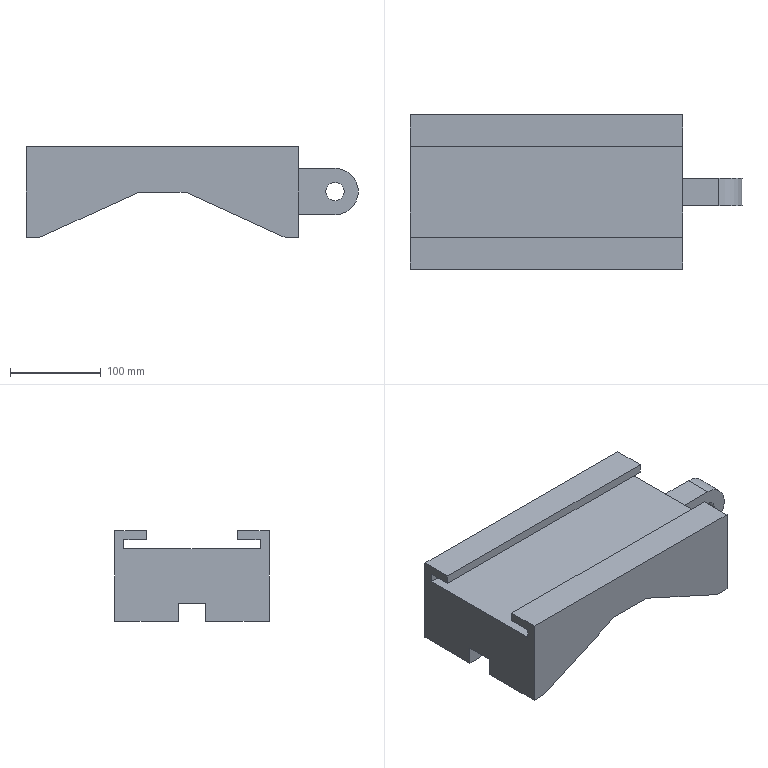Part | SolidWorks | features ICE 5, MirrorPattern 2, Extrusion 1 | 1 solid | 37 faces | box 365.5 x 170 x 100 mm | volume 2892418 mm3 | plane 34 | cylinder 3 | commonest cylinder face diameters 20 x2 51 x1
STEP:
#1=CARTESIAN_POINT('',(190.,15.,-29.5));
#2=VERTEX_POINT('',#1);
#3=CARTESIAN_POINT('',(190.,15.,-9.5));
#4=VERTEX_POINT('',#3);
#5=CARTESIAN_POINT('',(190.,15.,-19.5));
#6=DIRECTION('',(0.,1.,0.));
#7=DIRECTION('',(0.,0.,1.));
#8=AXIS2_PLACEMENT_3D('',#5,#6,#7);
#9=CIRCLE('',#8,10.);
#10=EDGE_CURVE('',#2,#4,#9,.T.);
#11=ORIENTED_EDGE('',*,*,#10,.T.);
#12=CARTESIAN_POINT('',(190.,-15.,-9.5));
#13=VERTEX_POINT('',#12);
#14=CARTESIAN_POINT('',(190.,15.,-9.5));
#15=DIRECTION('',(0.,-1.,0.));
#16=VECTOR('',#15,1000.);
#17=LINE('',#14,#16);
#18=EDGE_CURVE('',#4,#13,#17,.T.);
#19=ORIENTED_EDGE('',*,*,#18,.T.);
#20=CARTESIAN_POINT('',(190.,-15.,-29.5));
#21=VERTEX_POINT('',#20);
#22=CARTESIAN_POINT('',(190.,-15.,-19.5));
#23=DIRECTION('',(0.,1.,0.));
#24=DIRECTION('',(0.,0.,1.));
#25=AXIS2_PLACEMENT_3D('',#22,#23,#24);
#26=CIRCLE('',#25,10.);
#27=EDGE_CURVE('',#21,#13,#26,.T.);
#28=ORIENTED_EDGE('',*,*,#27,.F.);
#29=CARTESIAN_POINT('',(190.,15.,-29.5));
#30=DIRECTION('',(0.,-1.,0.));
#31=VECTOR('',#30,1000.);
#32=LINE('',#29,#31);
#33=EDGE_CURVE('',#2,#21,#32,.T.);
#34=ORIENTED_EDGE('',*,*,#33,.F.);
#35=EDGE_LOOP('',(#11,#19,#28,#34));
#36=FACE_OUTER_BOUND('',#35,.T.);
#37=CARTESIAN_POINT('',(190.,15.,-19.5));
#38=DIRECTION('',(0.,-1.,0.));
#39=DIRECTION('',(0.,0.,-1.));
#40=AXIS2_PLACEMENT_3D('',#37,#38,#39);
#41=CYLINDRICAL_SURFACE('',#40,10.);
#42=ADVANCED_FACE('',(#36),#41,.F.);
#43=CARTESIAN_POINT('',(150.,-15.,-70.));
#44=VERTEX_POINT('',#43);
#45=CARTESIAN_POINT('',(150.,-85.,-70.));
#46=VERTEX_POINT('',#45);
#47=CARTESIAN_POINT('',(150.,85.,-70.));
#48=DIRECTION('',(0.,-1.,0.));
#49=VECTOR('',#48,1000.);
#50=LINE('',#47,#49);
#51=EDGE_CURVE('',#44,#46,#50,.T.);
#52=ORIENTED_EDGE('',*,*,#51,.F.);
#53=CARTESIAN_POINT('',(150.,-15.,-50.));
#54=VERTEX_POINT('',#53);
#55=CARTESIAN_POINT('',(150.,-15.,-50.));
#56=DIRECTION('',(0.,0.,1.));
#57=VECTOR('',#56,1000.);
#58=LINE('',#55,#57);
#59=EDGE_CURVE('',#44,#54,#58,.T.);
#60=ORIENTED_EDGE('',*,*,#59,.T.);
#61=CARTESIAN_POINT('',(150.,15.,-50.));
#62=VERTEX_POINT('',#61);
#63=CARTESIAN_POINT('',(150.,-15.,-50.));
#64=DIRECTION('',(0.,1.,0.));
#65=VECTOR('',#64,1000.);
#66=LINE('',#63,#65);
#67=EDGE_CURVE('',#54,#62,#66,.T.);
#68=ORIENTED_EDGE('',*,*,#67,.T.);
#69=CARTESIAN_POINT('',(150.,15.,-70.));
#70=VERTEX_POINT('',#69);
#71=CARTESIAN_POINT('',(150.,15.,-50.));
#72=DIRECTION('',(0.,0.,1.));
#73=VECTOR('',#72,1000.);
#74=LINE('',#71,#73);
#75=EDGE_CURVE('',#70,#62,#74,.T.);
#76=ORIENTED_EDGE('',*,*,#75,.F.);
#77=CARTESIAN_POINT('',(150.,85.,-70.));
#78=VERTEX_POINT('',#77);
#79=CARTESIAN_POINT('',(150.,85.,-70.));
#80=DIRECTION('',(0.,-1.,0.));
#81=VECTOR('',#80,1000.);
#82=LINE('',#79,#81);
#83=EDGE_CURVE('',#78,#70,#82,.T.);
#84=ORIENTED_EDGE('',*,*,#83,.F.);
#85=CARTESIAN_POINT('',(150.,85.,30.));
#86=VERTEX_POINT('',#85);
#87=CARTESIAN_POINT('',(150.,85.,10.));
#88=DIRECTION('',(0.,0.,-1.));
#89=VECTOR('',#88,1000.);
#90=LINE('',#87,#89);
#91=EDGE_CURVE('',#86,#78,#90,.T.);
#92=ORIENTED_EDGE('',*,*,#91,.F.);
#93=CARTESIAN_POINT('',(150.,50.,30.));
#94=VERTEX_POINT('',#93);
#95=CARTESIAN_POINT('',(150.,85.,30.));
#96=DIRECTION('',(0.,1.,0.));
#97=VECTOR('',#96,1000.);
#98=LINE('',#95,#97);
#99=EDGE_CURVE('',#94,#86,#98,.T.);
#100=ORIENTED_EDGE('',*,*,#99,.F.);
#101=CARTESIAN_POINT('',(150.,50.,20.));
#102=VERTEX_POINT('',#101);
#103=CARTESIAN_POINT('',(150.,50.,30.));
#104=DIRECTION('',(0.,0.,1.));
#105=VECTOR('',#104,1000.);
#106=LINE('',#103,#105);
#107=EDGE_CURVE('',#102,#94,#106,.T.);
#108=ORIENTED_EDGE('',*,*,#107,.F.);
#109=CARTESIAN_POINT('',(150.,75.,20.));
#110=VERTEX_POINT('',#109);
#111=CARTESIAN_POINT('',(150.,50.,20.));
#112=DIRECTION('',(0.,1.,0.));
#113=VECTOR('',#112,1000.);
#114=LINE('',#111,#113);
#115=EDGE_CURVE('',#102,#110,#114,.T.);
#116=ORIENTED_EDGE('',*,*,#115,.T.);
#117=CARTESIAN_POINT('',(150.,75.,10.));
#118=VERTEX_POINT('',#117);
#119=CARTESIAN_POINT('',(150.,75.,30.));
#120=DIRECTION('',(0.,0.,-1.));
#121=VECTOR('',#120,1000.);
#122=LINE('',#119,#121);
#123=EDGE_CURVE('',#110,#118,#122,.T.);
#124=ORIENTED_EDGE('',*,*,#123,.T.);
#125=CARTESIAN_POINT('',(150.,-75.,10.));
#126=VERTEX_POINT('',#125);
#127=CARTESIAN_POINT('',(150.,85.,10.));
#128=DIRECTION('',(0.,1.,0.));
#129=VECTOR('',#128,1000.);
#130=LINE('',#127,#129);
#131=EDGE_CURVE('',#126,#118,#130,.T.);
#132=ORIENTED_EDGE('',*,*,#131,.F.);
#133=CARTESIAN_POINT('',(150.,-75.,20.));
#134=VERTEX_POINT('',#133);
#135=CARTESIAN_POINT('',(150.,-75.,30.));
#136=DIRECTION('',(0.,0.,-1.));
#137=VECTOR('',#136,1000.);
#138=LINE('',#135,#137);
#139=EDGE_CURVE('',#134,#126,#138,.T.);
#140=ORIENTED_EDGE('',*,*,#139,.F.);
#141=CARTESIAN_POINT('',(150.,-50.,20.));
#142=VERTEX_POINT('',#141);
#143=CARTESIAN_POINT('',(150.,-50.,20.));
#144=DIRECTION('',(0.,-1.,0.));
#145=VECTOR('',#144,1000.);
#146=LINE('',#143,#145);
#147=EDGE_CURVE('',#142,#134,#146,.T.);
#148=ORIENTED_EDGE('',*,*,#147,.F.);
#149=CARTESIAN_POINT('',(150.,-50.,30.));
#150=VERTEX_POINT('',#149);
#151=CARTESIAN_POINT('',(150.,-50.,30.));
#152=DIRECTION('',(0.,0.,1.));
#153=VECTOR('',#152,1000.);
#154=LINE('',#151,#153);
#155=EDGE_CURVE('',#142,#150,#154,.T.);
#156=ORIENTED_EDGE('',*,*,#155,.T.);
#157=CARTESIAN_POINT('',(150.,-85.,30.));
#158=VERTEX_POINT('',#157);
#159=CARTESIAN_POINT('',(150.,-85.,30.));
#160=DIRECTION('',(0.,1.,0.));
#161=VECTOR('',#160,1000.);
#162=LINE('',#159,#161);
#163=EDGE_CURVE('',#158,#150,#162,.T.);
#164=ORIENTED_EDGE('',*,*,#163,.F.);
#165=CARTESIAN_POINT('',(150.,-85.,10.));
#166=DIRECTION('',(0.,0.,-1.));
#167=VECTOR('',#166,1000.);
#168=LINE('',#165,#167);
#169=EDGE_CURVE('',#158,#46,#168,.T.);
#170=ORIENTED_EDGE('',*,*,#169,.T.);
#171=EDGE_LOOP('',(#52,#60,#68,#76,#84,#92,#100,#108,#116,#124,#132,#140,#148,#156,#164,#170));
#172=FACE_OUTER_BOUND('',#171,.T.);
#173=CARTESIAN_POINT('',(150.,15.,6.));
#174=VERTEX_POINT('',#173);
#175=CARTESIAN_POINT('',(150.,-15.,6.));
#176=VERTEX_POINT('',#175);
#177=CARTESIAN_POINT('',(150.,15.,6.));
#178=DIRECTION('',(0.,-1.,0.));
#179=VECTOR('',#178,1000.);
#180=LINE('',#177,#179);
#181=EDGE_CURVE('',#174,#176,#180,.T.);
#182=ORIENTED_EDGE('',*,*,#181,.F.);
#183=CARTESIAN_POINT('',(150.,15.,-45.));
#184=VERTEX_POINT('',#183);
#185=CARTESIAN_POINT('',(150.,15.,6.));
#186=DIRECTION('',(0.,0.,1.));
#187=VECTOR('',#186,1000.);
#188=LINE('',#185,#187);
#189=EDGE_CURVE('',#184,#174,#188,.T.);
#190=ORIENTED_EDGE('',*,*,#189,.F.);
#191=CARTESIAN_POINT('',(150.,-15.,-45.));
#192=VERTEX_POINT('',#191);
#193=CARTESIAN_POINT('',(150.,15.,-45.));
#194=DIRECTION('',(0.,-1.,0.));
#195=VECTOR('',#194,1000.);
#196=LINE('',#193,#195);
#197=EDGE_CURVE('',#184,#192,#196,.T.);
#198=ORIENTED_EDGE('',*,*,#197,.T.);
#199=CARTESIAN_POINT('',(150.,-15.,6.));
#200=DIRECTION('',(0.,0.,1.));
#201=VECTOR('',#200,1000.);
#202=LINE('',#199,#201);
#203=EDGE_CURVE('',#192,#176,#202,.T.);
#204=ORIENTED_EDGE('',*,*,#203,.T.);
#205=EDGE_LOOP('',(#182,#190,#198,#204));
#206=FACE_BOUND('',#205,.T.);
#207=CARTESIAN_POINT('',(150.,85.,10.));
#208=DIRECTION('',(-1.,0.,0.));
#209=DIRECTION('',(0.,-1.,0.));
#210=AXIS2_PLACEMENT_3D('',#207,#208,#209);
#211=PLANE('',#210);
#212=ADVANCED_FACE('',(#172,#206),#211,.F.);
#213=CARTESIAN_POINT('',(25.,85.,-20.));
#214=VERTEX_POINT('',#213);
#215=CARTESIAN_POINT('',(25.,15.,-20.));
#216=VERTEX_POINT('',#215);
#217=CARTESIAN_POINT('',(25.,85.,-20.));
#218=DIRECTION('',(0.,-1.,0.));
#219=VECTOR('',#218,1000.);
#220=LINE('',#217,#219);
#221=EDGE_CURVE('',#214,#216,#220,.T.);
#222=ORIENTED_EDGE('',*,*,#221,.T.);
#223=CARTESIAN_POINT('',(-25.,15.,-20.));
#224=VERTEX_POINT('',#223);
#225=CARTESIAN_POINT('',(-25.,15.,-20.));
#226=DIRECTION('',(-1.,0.,0.));
#227=VECTOR('',#226,1000.);
#228=LINE('',#225,#227);
#229=EDGE_CURVE('',#216,#224,#228,.T.);
#230=ORIENTED_EDGE('',*,*,#229,.T.);
#231=CARTESIAN_POINT('',(-25.,85.,-20.));
#232=VERTEX_POINT('',#231);
#233=CARTESIAN_POINT('',(-25.,85.,-20.));
#234=DIRECTION('',(0.,-1.,0.));
#235=VECTOR('',#234,1000.);
#236=LINE('',#233,#235);
#237=EDGE_CURVE('',#232,#224,#236,.T.);
#238=ORIENTED_EDGE('',*,*,#237,.F.);
#239=CARTESIAN_POINT('',(-25.,85.,-20.));
#240=DIRECTION('',(-1.,0.,0.));
#241=VECTOR('',#240,1000.);
#242=LINE('',#239,#241);
#243=EDGE_CURVE('',#214,#232,#242,.T.);
#244=ORIENTED_EDGE('',*,*,#243,.F.);
#245=EDGE_LOOP('',(#222,#230,#238,#244));
#246=FACE_OUTER_BOUND('',#245,.T.);
#247=CARTESIAN_POINT('',(-25.,85.,-20.));
#248=DIRECTION('',(0.,0.,1.));
#249=DIRECTION('',(1.,0.,0.));
#250=AXIS2_PLACEMENT_3D('',#247,#248,#249);
#251=PLANE('',#250);
#252=ADVANCED_FACE('',(#246),#251,.F.);
#253=ORIENTED_EDGE('',*,*,#83,.T.);
#254=CARTESIAN_POINT('',(135.,15.,-70.));
#255=VERTEX_POINT('',#254);
#256=CARTESIAN_POINT('',(150.,15.,-70.));
#257=DIRECTION('',(1.,0.,0.));
#258=VECTOR('',#257,1000.);
#259=LINE('',#256,#258);
#260=EDGE_CURVE('',#255,#70,#259,.T.);
#261=ORIENTED_EDGE('',*,*,#260,.F.);
#262=CARTESIAN_POINT('',(135.,85.,-70.));
#263=VERTEX_POINT('',#262);
#264=CARTESIAN_POINT('',(135.,85.,-70.));
#265=DIRECTION('',(0.,-1.,0.));
#266=VECTOR('',#265,1000.);
#267=LINE('',#264,#266);
#268=EDGE_CURVE('',#263,#255,#267,.T.);
#269=ORIENTED_EDGE('',*,*,#268,.F.);
#270=CARTESIAN_POINT('',(150.,85.,-70.));
#271=DIRECTION('',(1.,0.,0.));
#272=VECTOR('',#271,1000.);
#273=LINE('',#270,#272);
#274=EDGE_CURVE('',#263,#78,#273,.T.);
#275=ORIENTED_EDGE('',*,*,#274,.T.);
#276=EDGE_LOOP('',(#253,#261,#269,#275));
#277=FACE_OUTER_BOUND('',#276,.T.);
#278=CARTESIAN_POINT('',(150.,85.,-70.));
#279=DIRECTION('',(0.,0.,-1.));
#280=DIRECTION('',(-1.,0.,0.));
#281=AXIS2_PLACEMENT_3D('',#278,#279,#280);
#282=PLANE('',#281);
#283=ADVANCED_FACE('',(#277),#282,.T.);
#284=ORIENTED_EDGE('',*,*,#268,.T.);
#285=CARTESIAN_POINT('',(135.,15.,-70.));
#286=DIRECTION('',(0.9104,0.,-0.4138));
#287=VECTOR('',#286,1000.);
#288=LINE('',#285,#287);
#289=EDGE_CURVE('',#216,#255,#288,.T.);
#290=ORIENTED_EDGE('',*,*,#289,.F.);
#291=ORIENTED_EDGE('',*,*,#221,.F.);
#292=CARTESIAN_POINT('',(135.,85.,-70.));
#293=DIRECTION('',(0.9104,0.,-0.4138));
#294=VECTOR('',#293,1000.);
#295=LINE('',#292,#294);
#296=EDGE_CURVE('',#214,#263,#295,.T.);
#297=ORIENTED_EDGE('',*,*,#296,.T.);
#298=EDGE_LOOP('',(#284,#290,#291,#297));
#299=FACE_OUTER_BOUND('',#298,.T.);
#300=CARTESIAN_POINT('',(135.,85.,-70.));
#301=DIRECTION('',(-0.4138,0.,-0.9104));
#302=DIRECTION('',(-0.9104,0.,0.4138));
#303=AXIS2_PLACEMENT_3D('',#300,#301,#302);
#304=PLANE('',#303);
#305=ADVANCED_FACE('',(#299),#304,.T.);
#306=CARTESIAN_POINT('',(-135.,15.,-70.));
#307=VERTEX_POINT('',#306);
#308=CARTESIAN_POINT('',(-135.,15.,-70.));
#309=DIRECTION('',(-0.9104,0.,-0.4138));
#310=VECTOR('',#309,1000.);
#311=LINE('',#308,#310);
#312=EDGE_CURVE('',#224,#307,#311,.T.);
#313=ORIENTED_EDGE('',*,*,#312,.T.);
#314=CARTESIAN_POINT('',(-135.,85.,-70.));
#315=VERTEX_POINT('',#314);
#316=CARTESIAN_POINT('',(-135.,85.,-70.));
#317=DIRECTION('',(0.,-1.,0.));
#318=VECTOR('',#317,1000.);
#319=LINE('',#316,#318);
#320=EDGE_CURVE('',#315,#307,#319,.T.);
#321=ORIENTED_EDGE('',*,*,#320,.F.);
#322=CARTESIAN_POINT('',(-135.,85.,-70.));
#323=DIRECTION('',(-0.9104,0.,-0.4138));
#324=VECTOR('',#323,1000.);
#325=LINE('',#322,#324);
#326=EDGE_CURVE('',#232,#315,#325,.T.);
#327=ORIENTED_EDGE('',*,*,#326,.F.);
#328=ORIENTED_EDGE('',*,*,#237,.T.);
#329=EDGE_LOOP('',(#313,#321,#327,#328));
#330=FACE_OUTER_BOUND('',#329,.T.);
#331=CARTESIAN_POINT('',(-135.,85.,-70.));
#332=DIRECTION('',(-0.4138,0.,0.9104));
#333=DIRECTION('',(0.9104,0.,0.4138));
#334=AXIS2_PLACEMENT_3D('',#331,#332,#333);
#335=PLANE('',#334);
#336=ADVANCED_FACE('',(#330),#335,.F.);
#337=CARTESIAN_POINT('',(-150.,15.,-70.));
#338=VERTEX_POINT('',#337);
#339=CARTESIAN_POINT('',(-150.,15.,-70.));
#340=DIRECTION('',(-1.,0.,0.));
#341=VECTOR('',#340,1000.);
#342=LINE('',#339,#341);
#343=EDGE_CURVE('',#307,#338,#342,.T.);
#344=ORIENTED_EDGE('',*,*,#343,.T.);
#345=CARTESIAN_POINT('',(-150.,85.,-70.));
#346=VERTEX_POINT('',#345);
#347=CARTESIAN_POINT('',(-150.,85.,-70.));
#348=DIRECTION('',(0.,-1.,0.));
#349=VECTOR('',#348,1000.);
#350=LINE('',#347,#349);
#351=EDGE_CURVE('',#346,#338,#350,.T.);
#352=ORIENTED_EDGE('',*,*,#351,.F.);
#353=CARTESIAN_POINT('',(-150.,85.,-70.));
#354=DIRECTION('',(-1.,0.,0.));
#355=VECTOR('',#354,1000.);
#356=LINE('',#353,#355);
#357=EDGE_CURVE('',#315,#346,#356,.T.);
#358=ORIENTED_EDGE('',*,*,#357,.F.);
#359=ORIENTED_EDGE('',*,*,#320,.T.);
#360=EDGE_LOOP('',(#344,#352,#358,#359));
#361=FACE_OUTER_BOUND('',#360,.T.);
#362=CARTESIAN_POINT('',(-150.,85.,-70.));
#363=DIRECTION('',(0.,0.,1.));
#364=DIRECTION('',(1.,0.,0.));
#365=AXIS2_PLACEMENT_3D('',#362,#363,#364);
#366=PLANE('',#365);
#367=ADVANCED_FACE('',(#361),#366,.F.);
#368=CARTESIAN_POINT('',(-25.,15.,0.));
#369=VERTEX_POINT('',#368);
#370=CARTESIAN_POINT('',(25.,15.,0.));
#371=VERTEX_POINT('',#370);
#372=CARTESIAN_POINT('',(0.,15.,0.));
#373=DIRECTION('',(1.,0.,0.));
#374=VECTOR('',#373,1000.);
#375=LINE('',#372,#374);
#376=EDGE_CURVE('',#369,#371,#375,.T.);
#377=ORIENTED_EDGE('',*,*,#376,.T.);
#378=CARTESIAN_POINT('',(25.,-15.,0.));
#379=VERTEX_POINT('',#378);
#380=CARTESIAN_POINT('',(25.,-15.,0.));
#381=DIRECTION('',(0.,1.,0.));
#382=VECTOR('',#381,1000.);
#383=LINE('',#380,#382);
#384=EDGE_CURVE('',#379,#371,#383,.T.);
#385=ORIENTED_EDGE('',*,*,#384,.F.);
#386=CARTESIAN_POINT('',(-25.,-15.,0.));
#387=VERTEX_POINT('',#386);
#388=CARTESIAN_POINT('',(0.,-15.,0.));
#389=DIRECTION('',(1.,0.,0.));
#390=VECTOR('',#389,1000.);
#391=LINE('',#388,#390);
#392=EDGE_CURVE('',#387,#379,#391,.T.);
#393=ORIENTED_EDGE('',*,*,#392,.F.);
#394=CARTESIAN_POINT('',(-25.,-15.,0.));
#395=DIRECTION('',(0.,1.,0.));
#396=VECTOR('',#395,1000.);
#397=LINE('',#394,#396);
#398=EDGE_CURVE('',#387,#369,#397,.T.);
#399=ORIENTED_EDGE('',*,*,#398,.T.);
#400=EDGE_LOOP('',(#377,#385,#393,#399));
#401=FACE_OUTER_BOUND('',#400,.T.);
#402=CARTESIAN_POINT('',(0.,0.,0.));
#403=DIRECTION('',(0.,0.,1.));
#404=DIRECTION('',(1.,0.,0.));
#405=AXIS2_PLACEMENT_3D('',#402,#403,#404);
#406=PLANE('',#405);
#407=ADVANCED_FACE('',(#401),#406,.F.);
#408=CARTESIAN_POINT('',(-150.,75.,20.));
#409=VERTEX_POINT('',#408);
#410=CARTESIAN_POINT('',(-150.,75.,20.));
#411=DIRECTION('',(1.,0.,0.));
#412=VECTOR('',#411,1000.);
#413=LINE('',#410,#412);
#414=EDGE_CURVE('',#409,#110,#413,.T.);
#415=ORIENTED_EDGE('',*,*,#414,.F.);
#416=CARTESIAN_POINT('',(-150.,75.,10.));
#417=VERTEX_POINT('',#416);
#418=CARTESIAN_POINT('',(-150.,75.,30.));
#419=DIRECTION('',(0.,0.,-1.));
#420=VECTOR('',#419,1000.);
#421=LINE('',#418,#420);
#422=EDGE_CURVE('',#409,#417,#421,.T.);
#423=ORIENTED_EDGE('',*,*,#422,.T.);
#424=CARTESIAN_POINT('',(-150.,75.,10.));
#425=DIRECTION('',(1.,0.,0.));
#426=VECTOR('',#425,1000.);
#427=LINE('',#424,#426);
#428=EDGE_CURVE('',#417,#118,#427,.T.);
#429=ORIENTED_EDGE('',*,*,#428,.T.);
#430=ORIENTED_EDGE('',*,*,#123,.F.);
#431=EDGE_LOOP('',(#415,#423,#429,#430));
#432=FACE_OUTER_BOUND('',#431,.T.);
#433=CARTESIAN_POINT('',(-150.,75.,30.));
#434=DIRECTION('',(0.,1.,0.));
#435=DIRECTION('',(-1.,0.,0.));
#436=AXIS2_PLACEMENT_3D('',#433,#434,#435);
#437=PLANE('',#436);
#438=ADVANCED_FACE('',(#432),#437,.F.);
#439=CARTESIAN_POINT('',(-150.,-75.,10.));
#440=VERTEX_POINT('',#439);
#441=CARTESIAN_POINT('',(-150.,85.,10.));
#442=DIRECTION('',(0.,-1.,0.));
#443=VECTOR('',#442,1000.);
#444=LINE('',#441,#443);
#445=EDGE_CURVE('',#417,#440,#444,.T.);
#446=ORIENTED_EDGE('',*,*,#445,.T.);
#447=CARTESIAN_POINT('',(-150.,-75.,10.));
#448=DIRECTION('',(-1.,0.,0.));
#449=VECTOR('',#448,1000.);
#450=LINE('',#447,#449);
#451=EDGE_CURVE('',#126,#440,#450,.T.);
#452=ORIENTED_EDGE('',*,*,#451,.F.);
#453=ORIENTED_EDGE('',*,*,#131,.T.);
#454=ORIENTED_EDGE('',*,*,#428,.F.);
#455=EDGE_LOOP('',(#446,#452,#453,#454));
#456=FACE_OUTER_BOUND('',#455,.T.);
#457=CARTESIAN_POINT('',(0.,0.,10.));
#458=DIRECTION('',(0.,0.,1.));
#459=DIRECTION('',(1.,0.,0.));
#460=AXIS2_PLACEMENT_3D('',#457,#458,#459);
#461=PLANE('',#460);
#462=ADVANCED_FACE('',(#456),#461,.T.);
#463=ORIENTED_EDGE('',*,*,#91,.T.);
#464=ORIENTED_EDGE('',*,*,#274,.F.);
#465=ORIENTED_EDGE('',*,*,#296,.F.);
#466=ORIENTED_EDGE('',*,*,#243,.T.);
#467=ORIENTED_EDGE('',*,*,#326,.T.);
#468=ORIENTED_EDGE('',*,*,#357,.T.);
#469=CARTESIAN_POINT('',(-150.,85.,30.));
#470=VERTEX_POINT('',#469);
#471=CARTESIAN_POINT('',(-150.,85.,10.));
#472=DIRECTION('',(0.,0.,-1.));
#473=VECTOR('',#472,1000.);
#474=LINE('',#471,#473);
#475=EDGE_CURVE('',#470,#346,#474,.T.);
#476=ORIENTED_EDGE('',*,*,#475,.F.);
#477=CARTESIAN_POINT('',(-150.,85.,30.));
#478=DIRECTION('',(-1.,0.,0.));
#479=VECTOR('',#478,1000.);
#480=LINE('',#477,#479);
#481=EDGE_CURVE('',#86,#470,#480,.T.);
#482=ORIENTED_EDGE('',*,*,#481,.F.);
#483=EDGE_LOOP('',(#463,#464,#465,#466,#467,#468,#476,#482));
#484=FACE_OUTER_BOUND('',#483,.T.);
#485=CARTESIAN_POINT('',(-150.,85.,10.));
#486=DIRECTION('',(0.,-1.,0.));
#487=DIRECTION('',(0.,0.,-1.));
#488=AXIS2_PLACEMENT_3D('',#485,#486,#487);
#489=PLANE('',#488);
#490=ADVANCED_FACE('',(#484),#489,.F.);
#491=CARTESIAN_POINT('',(-150.,-15.,-50.));
#492=VERTEX_POINT('',#491);
#493=CARTESIAN_POINT('',(-150.,15.,-50.));
#494=VERTEX_POINT('',#493);
#495=CARTESIAN_POINT('',(-150.,-15.,-50.));
#496=DIRECTION('',(0.,1.,0.));
#497=VECTOR('',#496,1000.);
#498=LINE('',#495,#497);
#499=EDGE_CURVE('',#492,#494,#498,.T.);
#500=ORIENTED_EDGE('',*,*,#499,.F.);
#501=CARTESIAN_POINT('',(-150.,-15.,-70.));
#502=VERTEX_POINT('',#501);
#503=CARTESIAN_POINT('',(-150.,-15.,-50.));
#504=DIRECTION('',(0.,0.,1.));
#505=VECTOR('',#504,1000.);
#506=LINE('',#503,#505);
#507=EDGE_CURVE('',#502,#492,#506,.T.);
#508=ORIENTED_EDGE('',*,*,#507,.F.);
#509=CARTESIAN_POINT('',(-150.,-85.,-70.));
#510=VERTEX_POINT('',#509);
#511=CARTESIAN_POINT('',(-150.,85.,-70.));
#512=DIRECTION('',(0.,-1.,0.));
#513=VECTOR('',#512,1000.);
#514=LINE('',#511,#513);
#515=EDGE_CURVE('',#502,#510,#514,.T.);
#516=ORIENTED_EDGE('',*,*,#515,.T.);
#517=CARTESIAN_POINT('',(-150.,-85.,30.));
#518=VERTEX_POINT('',#517);
#519=CARTESIAN_POINT('',(-150.,-85.,10.));
#520=DIRECTION('',(0.,0.,-1.));
#521=VECTOR('',#520,1000.);
#522=LINE('',#519,#521);
#523=EDGE_CURVE('',#518,#510,#522,.T.);
#524=ORIENTED_EDGE('',*,*,#523,.F.);
#525=CARTESIAN_POINT('',(-150.,-50.,30.));
#526=VERTEX_POINT('',#525);
#527=CARTESIAN_POINT('',(-150.,-85.,30.));
#528=DIRECTION('',(0.,-1.,0.));
#529=VECTOR('',#528,1000.);
#530=LINE('',#527,#529);
#531=EDGE_CURVE('',#526,#518,#530,.T.);
#532=ORIENTED_EDGE('',*,*,#531,.F.);
#533=CARTESIAN_POINT('',(-150.,-50.,20.));
#534=VERTEX_POINT('',#533);
#535=CARTESIAN_POINT('',(-150.,-50.,30.));
#536=DIRECTION('',(0.,0.,-1.));
#537=VECTOR('',#536,1000.);
#538=LINE('',#535,#537);
#539=EDGE_CURVE('',#526,#534,#538,.T.);
#540=ORIENTED_EDGE('',*,*,#539,.T.);
#541=CARTESIAN_POINT('',(-150.,-75.,20.));
#542=VERTEX_POINT('',#541);
#543=CARTESIAN_POINT('',(-150.,-50.,20.));
#544=DIRECTION('',(0.,-1.,0.));
#545=VECTOR('',#544,1000.);
#546=LINE('',#543,#545);
#547=EDGE_CURVE('',#534,#542,#546,.T.);
#548=ORIENTED_EDGE('',*,*,#547,.T.);
#549=CARTESIAN_POINT('',(-150.,-75.,30.));
#550=DIRECTION('',(0.,0.,-1.));
#551=VECTOR('',#550,1000.);
#552=LINE('',#549,#551);
#553=EDGE_CURVE('',#542,#440,#552,.T.);
#554=ORIENTED_EDGE('',*,*,#553,.T.);
#555=ORIENTED_EDGE('',*,*,#445,.F.);
#556=ORIENTED_EDGE('',*,*,#422,.F.);
#557=CARTESIAN_POINT('',(-150.,50.,20.));
#558=VERTEX_POINT('',#557);
#559=CARTESIAN_POINT('',(-150.,50.,20.));
#560=DIRECTION('',(0.,1.,0.));
#561=VECTOR('',#560,1000.);
#562=LINE('',#559,#561);
#563=EDGE_CURVE('',#558,#409,#562,.T.);
#564=ORIENTED_EDGE('',*,*,#563,.F.);
#565=CARTESIAN_POINT('',(-150.,50.,30.));
#566=VERTEX_POINT('',#565);
#567=CARTESIAN_POINT('',(-150.,50.,30.));
#568=DIRECTION('',(0.,0.,-1.));
#569=VECTOR('',#568,1000.);
#570=LINE('',#567,#569);
#571=EDGE_CURVE('',#566,#558,#570,.T.);
#572=ORIENTED_EDGE('',*,*,#571,.F.);
#573=CARTESIAN_POINT('',(-150.,85.,30.));
#574=DIRECTION('',(0.,-1.,0.));
#575=VECTOR('',#574,1000.);
#576=LINE('',#573,#575);
#577=EDGE_CURVE('',#470,#566,#576,.T.);
#578=ORIENTED_EDGE('',*,*,#577,.F.);
#579=ORIENTED_EDGE('',*,*,#475,.T.);
#580=ORIENTED_EDGE('',*,*,#351,.T.);
#581=CARTESIAN_POINT('',(-150.,15.,-50.));
#582=DIRECTION('',(0.,0.,1.));
#583=VECTOR('',#582,1000.);
#584=LINE('',#581,#583);
#585=EDGE_CURVE('',#338,#494,#584,.T.);
#586=ORIENTED_EDGE('',*,*,#585,.T.);
#587=EDGE_LOOP('',(#500,#508,#516,#524,#532,#540,#548,#554,#555,#556,#564,#572,#578,#579,#580,#586));
#588=FACE_OUTER_BOUND('',#587,.T.);
#589=CARTESIAN_POINT('',(-150.,85.,10.));
#590=DIRECTION('',(1.,0.,0.));
#591=DIRECTION('',(0.,1.,0.));
#592=AXIS2_PLACEMENT_3D('',#589,#590,#591);
#593=PLANE('',#592);
#594=ADVANCED_FACE('',(#588),#593,.F.);
#595=CARTESIAN_POINT('',(135.,-85.,-70.));
#596=VERTEX_POINT('',#595);
#597=CARTESIAN_POINT('',(150.,-85.,-70.));
#598=DIRECTION('',(1.,0.,0.));
#599=VECTOR('',#598,1000.);
#600=LINE('',#597,#599);
#601=EDGE_CURVE('',#596,#46,#600,.T.);
#602=ORIENTED_EDGE('',*,*,#601,.T.);
#603=ORIENTED_EDGE('',*,*,#169,.F.);
#604=CARTESIAN_POINT('',(-150.,-85.,30.));
#605=DIRECTION('',(1.,0.,0.));
#606=VECTOR('',#605,1000.);
#607=LINE('',#604,#606);
#608=EDGE_CURVE('',#518,#158,#607,.T.);
#609=ORIENTED_EDGE('',*,*,#608,.F.);
#610=ORIENTED_EDGE('',*,*,#523,.T.);
#611=CARTESIAN_POINT('',(-135.,-85.,-70.));
#612=VERTEX_POINT('',#611);
#613=CARTESIAN_POINT('',(-150.,-85.,-70.));
#614=DIRECTION('',(-1.,0.,0.));
#615=VECTOR('',#614,1000.);
#616=LINE('',#613,#615);
#617=EDGE_CURVE('',#612,#510,#616,.T.);
#618=ORIENTED_EDGE('',*,*,#617,.F.);
#619=CARTESIAN_POINT('',(-25.,-85.,-20.));
#620=VERTEX_POINT('',#619);
#621=CARTESIAN_POINT('',(-135.,-85.,-70.));
#622=DIRECTION('',(-0.9104,0.,-0.4138));
#623=VECTOR('',#622,1000.);
#624=LINE('',#621,#623);
#625=EDGE_CURVE('',#620,#612,#624,.T.);
#626=ORIENTED_EDGE('',*,*,#625,.F.);
#627=CARTESIAN_POINT('',(25.,-85.,-20.));
#628=VERTEX_POINT('',#627);
#629=CARTESIAN_POINT('',(-25.,-85.,-20.));
#630=DIRECTION('',(-1.,0.,0.));
#631=VECTOR('',#630,1000.);
#632=LINE('',#629,#631);
#633=EDGE_CURVE('',#628,#620,#632,.T.);
#634=ORIENTED_EDGE('',*,*,#633,.F.);
#635=CARTESIAN_POINT('',(135.,-85.,-70.));
#636=DIRECTION('',(0.9104,0.,-0.4138));
#637=VECTOR('',#636,1000.);
#638=LINE('',#635,#637);
#639=EDGE_CURVE('',#628,#596,#638,.T.);
#640=ORIENTED_EDGE('',*,*,#639,.T.);
#641=EDGE_LOOP('',(#602,#603,#609,#610,#618,#626,#634,#640));
#642=FACE_OUTER_BOUND('',#641,.T.);
#643=CARTESIAN_POINT('',(-150.,-85.,10.));
#644=DIRECTION('',(0.,1.,0.));
#645=DIRECTION('',(0.,0.,1.));
#646=AXIS2_PLACEMENT_3D('',#643,#644,#645);
#647=PLANE('',#646);
#648=ADVANCED_FACE('',(#642),#647,.F.);
#649=ORIENTED_EDGE('',*,*,#577,.T.);
#650=CARTESIAN_POINT('',(-150.,50.,30.));
#651=DIRECTION('',(-1.,0.,0.));
#652=VECTOR('',#651,1000.);
#653=LINE('',#650,#652);
#654=EDGE_CURVE('',#94,#566,#653,.T.);
#655=ORIENTED_EDGE('',*,*,#654,.F.);
#656=ORIENTED_EDGE('',*,*,#99,.T.);
#657=ORIENTED_EDGE('',*,*,#481,.T.);
#658=EDGE_LOOP('',(#649,#655,#656,#657));
#659=FACE_OUTER_BOUND('',#658,.T.);
#660=CARTESIAN_POINT('',(0.,0.,30.));
#661=DIRECTION('',(0.,0.,1.));
#662=DIRECTION('',(1.,0.,0.));
#663=AXIS2_PLACEMENT_3D('',#660,#661,#662);
#664=PLANE('',#663);
#665=ADVANCED_FACE('',(#659),#664,.T.);
#666=ORIENTED_EDGE('',*,*,#553,.F.);
#667=CARTESIAN_POINT('',(-150.,-75.,20.));
#668=DIRECTION('',(1.,0.,0.));
#669=VECTOR('',#668,1000.);
#670=LINE('',#667,#669);
#671=EDGE_CURVE('',#542,#134,#670,.T.);
#672=ORIENTED_EDGE('',*,*,#671,.T.);
#673=ORIENTED_EDGE('',*,*,#139,.T.);
#674=ORIENTED_EDGE('',*,*,#451,.T.);
#675=EDGE_LOOP('',(#666,#672,#673,#674));
#676=FACE_OUTER_BOUND('',#675,.T.);
#677=CARTESIAN_POINT('',(-150.,-75.,30.));
#678=DIRECTION('',(0.,-1.,0.));
#679=DIRECTION('',(0.,0.,-1.));
#680=AXIS2_PLACEMENT_3D('',#677,#678,#679);
#681=PLANE('',#680);
#682=ADVANCED_FACE('',(#676),#681,.F.);
#683=ORIENTED_EDGE('',*,*,#531,.T.);
#684=ORIENTED_EDGE('',*,*,#608,.T.);
#685=ORIENTED_EDGE('',*,*,#163,.T.);
#686=CARTESIAN_POINT('',(-150.,-50.,30.));
#687=DIRECTION('',(-1.,0.,0.));
#688=VECTOR('',#687,1000.);
#689=LINE('',#686,#688);
#690=EDGE_CURVE('',#150,#526,#689,.T.);
#691=ORIENTED_EDGE('',*,*,#690,.T.);
#692=EDGE_LOOP('',(#683,#684,#685,#691));
#693=FACE_OUTER_BOUND('',#692,.T.);
#694=CARTESIAN_POINT('',(0.,0.,30.));
#695=DIRECTION('',(0.,0.,-1.));
#696=DIRECTION('',(-1.,0.,0.));
#697=AXIS2_PLACEMENT_3D('',#694,#695,#696);
#698=PLANE('',#697);
#699=ADVANCED_FACE('',(#693),#698,.F.);
#700=ORIENTED_EDGE('',*,*,#414,.T.);
#701=ORIENTED_EDGE('',*,*,#115,.F.);
#702=CARTESIAN_POINT('',(-150.,50.,20.));
#703=DIRECTION('',(1.,0.,0.));
#704=VECTOR('',#703,1000.);
#705=LINE('',#702,#704);
#706=EDGE_CURVE('',#558,#102,#705,.T.);
#707=ORIENTED_EDGE('',*,*,#706,.F.);
#708=ORIENTED_EDGE('',*,*,#563,.T.);
#709=EDGE_LOOP('',(#700,#701,#707,#708));
#710=FACE_OUTER_BOUND('',#709,.T.);
#711=CARTESIAN_POINT('',(-150.,50.,20.));
#712=DIRECTION('',(0.,0.,1.));
#713=DIRECTION('',(1.,0.,0.));
#714=AXIS2_PLACEMENT_3D('',#711,#712,#713);
#715=PLANE('',#714);
#716=ADVANCED_FACE('',(#710),#715,.F.);
#717=ORIENTED_EDGE('',*,*,#571,.T.);
#718=ORIENTED_EDGE('',*,*,#706,.T.);
#719=ORIENTED_EDGE('',*,*,#107,.T.);
#720=ORIENTED_EDGE('',*,*,#654,.T.);
#721=EDGE_LOOP('',(#717,#718,#719,#720));
#722=FACE_OUTER_BOUND('',#721,.T.);
#723=CARTESIAN_POINT('',(0.,50.,0.));
#724=DIRECTION('',(0.,-1.,0.));
#725=DIRECTION('',(1.,0.,0.));
#726=AXIS2_PLACEMENT_3D('',#723,#724,#725);
#727=PLANE('',#726);
#728=ADVANCED_FACE('',(#722),#727,.T.);
#729=ORIENTED_EDGE('',*,*,#671,.F.);
#730=ORIENTED_EDGE('',*,*,#547,.F.);
#731=CARTESIAN_POINT('',(-150.,-50.,20.));
#732=DIRECTION('',(1.,0.,0.));
#733=VECTOR('',#732,1000.);
#734=LINE('',#731,#733);
#735=EDGE_CURVE('',#534,#142,#734,.T.);
#736=ORIENTED_EDGE('',*,*,#735,.T.);
#737=ORIENTED_EDGE('',*,*,#147,.T.);
#738=EDGE_LOOP('',(#729,#730,#736,#737));
#739=FACE_OUTER_BOUND('',#738,.T.);
#740=CARTESIAN_POINT('',(-150.,-50.,20.));
#741=DIRECTION('',(0.,0.,-1.));
#742=DIRECTION('',(-1.,0.,0.));
#743=AXIS2_PLACEMENT_3D('',#740,#741,#742);
#744=PLANE('',#743);
#745=ADVANCED_FACE('',(#739),#744,.T.);
#746=ORIENTED_EDGE('',*,*,#539,.F.);
#747=ORIENTED_EDGE('',*,*,#690,.F.);
#748=ORIENTED_EDGE('',*,*,#155,.F.);
#749=ORIENTED_EDGE('',*,*,#735,.F.);
#750=EDGE_LOOP('',(#746,#747,#748,#749));
#751=FACE_OUTER_BOUND('',#750,.T.);
#752=CARTESIAN_POINT('',(0.,-50.,0.));
#753=DIRECTION('',(0.,1.,0.));
#754=DIRECTION('',(1.,0.,0.));
#755=AXIS2_PLACEMENT_3D('',#752,#753,#754);
#756=PLANE('',#755);
#757=ADVANCED_FACE('',(#751),#756,.T.);
#758=CARTESIAN_POINT('',(25.,-15.,-20.));
#759=VERTEX_POINT('',#758);
#760=CARTESIAN_POINT('',(-25.,-15.,-20.));
#761=VERTEX_POINT('',#760);
#762=CARTESIAN_POINT('',(-25.,-15.,-20.));
#763=DIRECTION('',(-1.,0.,0.));
#764=VECTOR('',#763,1000.);
#765=LINE('',#762,#764);
#766=EDGE_CURVE('',#759,#761,#765,.T.);
#767=ORIENTED_EDGE('',*,*,#766,.F.);
#768=CARTESIAN_POINT('',(25.,85.,-20.));
#769=DIRECTION('',(0.,-1.,0.));
#770=VECTOR('',#769,1000.);
#771=LINE('',#768,#770);
#772=EDGE_CURVE('',#759,#628,#771,.T.);
#773=ORIENTED_EDGE('',*,*,#772,.T.);
#774=ORIENTED_EDGE('',*,*,#633,.T.);
#775=CARTESIAN_POINT('',(-25.,85.,-20.));
#776=DIRECTION('',(0.,-1.,0.));
#777=VECTOR('',#776,1000.);
#778=LINE('',#775,#777);
#779=EDGE_CURVE('',#761,#620,#778,.T.);
#780=ORIENTED_EDGE('',*,*,#779,.F.);
#781=EDGE_LOOP('',(#767,#773,#774,#780));
#782=FACE_OUTER_BOUND('',#781,.T.);
#783=CARTESIAN_POINT('',(-25.,85.,-20.));
#784=DIRECTION('',(0.,0.,1.));
#785=DIRECTION('',(1.,0.,0.));
#786=AXIS2_PLACEMENT_3D('',#783,#784,#785);
#787=PLANE('',#786);
#788=ADVANCED_FACE('',(#782),#787,.F.);
#789=CARTESIAN_POINT('',(-135.,-15.,-70.));
#790=VERTEX_POINT('',#789);
#791=CARTESIAN_POINT('',(-135.,85.,-70.));
#792=DIRECTION('',(0.,-1.,0.));
#793=VECTOR('',#792,1000.);
#794=LINE('',#791,#793);
#795=EDGE_CURVE('',#790,#612,#794,.T.);
#796=ORIENTED_EDGE('',*,*,#795,.F.);
#797=CARTESIAN_POINT('',(-135.,-15.,-70.));
#798=DIRECTION('',(-0.9104,0.,-0.4138));
#799=VECTOR('',#798,1000.);
#800=LINE('',#797,#799);
#801=EDGE_CURVE('',#761,#790,#800,.T.);
#802=ORIENTED_EDGE('',*,*,#801,.F.);
#803=ORIENTED_EDGE('',*,*,#779,.T.);
#804=ORIENTED_EDGE('',*,*,#625,.T.);
#805=EDGE_LOOP('',(#796,#802,#803,#804));
#806=FACE_OUTER_BOUND('',#805,.T.);
#807=CARTESIAN_POINT('',(-135.,85.,-70.));
#808=DIRECTION('',(-0.4138,0.,0.9104));
#809=DIRECTION('',(0.9104,0.,0.4138));
#810=AXIS2_PLACEMENT_3D('',#807,#808,#809);
#811=PLANE('',#810);
#812=ADVANCED_FACE('',(#806),#811,.F.);
#813=ORIENTED_EDGE('',*,*,#515,.F.);
#814=CARTESIAN_POINT('',(-150.,-15.,-70.));
#815=DIRECTION('',(-1.,0.,0.));
#816=VECTOR('',#815,1000.);
#817=LINE('',#814,#816);
#818=EDGE_CURVE('',#790,#502,#817,.T.);
#819=ORIENTED_EDGE('',*,*,#818,.F.);
#820=ORIENTED_EDGE('',*,*,#795,.T.);
#821=ORIENTED_EDGE('',*,*,#617,.T.);
#822=EDGE_LOOP('',(#813,#819,#820,#821));
#823=FACE_OUTER_BOUND('',#822,.T.);
#824=CARTESIAN_POINT('',(-150.,85.,-70.));
#825=DIRECTION('',(0.,0.,1.));
#826=DIRECTION('',(1.,0.,0.));
#827=AXIS2_PLACEMENT_3D('',#824,#825,#826);
#828=PLANE('',#827);
#829=ADVANCED_FACE('',(#823),#828,.F.);
#830=CARTESIAN_POINT('',(-135.,15.,-50.));
#831=VERTEX_POINT('',#830);
#832=CARTESIAN_POINT('',(-25.,15.,0.));
#833=DIRECTION('',(0.9104,0.,0.4138));
#834=VECTOR('',#833,1000.);
#835=LINE('',#832,#834);
#836=EDGE_CURVE('',#831,#369,#835,.T.);
#837=ORIENTED_EDGE('',*,*,#836,.T.);
#838=ORIENTED_EDGE('',*,*,#398,.F.);
#839=CARTESIAN_POINT('',(-135.,-15.,-50.));
#840=VERTEX_POINT('',#839);
#841=CARTESIAN_POINT('',(-25.,-15.,0.));
#842=DIRECTION('',(0.9104,0.,0.4138));
#843=VECTOR('',#842,1000.);
#844=LINE('',#841,#843);
#845=EDGE_CURVE('',#840,#387,#844,.T.);
#846=ORIENTED_EDGE('',*,*,#845,.F.);
#847=CARTESIAN_POINT('',(-135.,-15.,-50.));
#848=DIRECTION('',(0.,1.,0.));
#849=VECTOR('',#848,1000.);
#850=LINE('',#847,#849);
#851=EDGE_CURVE('',#840,#831,#850,.T.);
#852=ORIENTED_EDGE('',*,*,#851,.T.);
#853=EDGE_LOOP('',(#837,#838,#846,#852));
#854=FACE_OUTER_BOUND('',#853,.T.);
#855=CARTESIAN_POINT('',(-25.,-15.,0.));
#856=DIRECTION('',(-0.4138,0.,0.9104));
#857=DIRECTION('',(0.9104,0.,0.4138));
#858=AXIS2_PLACEMENT_3D('',#855,#856,#857);
#859=PLANE('',#858);
#860=ADVANCED_FACE('',(#854),#859,.F.);
#861=CARTESIAN_POINT('',(-135.,15.,-50.));
#862=DIRECTION('',(1.,0.,0.));
#863=VECTOR('',#862,1000.);
#864=LINE('',#861,#863);
#865=EDGE_CURVE('',#494,#831,#864,.T.);
#866=ORIENTED_EDGE('',*,*,#865,.T.);
#867=ORIENTED_EDGE('',*,*,#851,.F.);
#868=CARTESIAN_POINT('',(-135.,-15.,-50.));
#869=DIRECTION('',(1.,0.,0.));
#870=VECTOR('',#869,1000.);
#871=LINE('',#868,#870);
#872=EDGE_CURVE('',#492,#840,#871,.T.);
#873=ORIENTED_EDGE('',*,*,#872,.F.);
#874=ORIENTED_EDGE('',*,*,#499,.T.);
#875=EDGE_LOOP('',(#866,#867,#873,#874));
#876=FACE_OUTER_BOUND('',#875,.T.);
#877=CARTESIAN_POINT('',(-135.,-15.,-50.));
#878=DIRECTION('',(0.,0.,1.));
#879=DIRECTION('',(1.,0.,0.));
#880=AXIS2_PLACEMENT_3D('',#877,#878,#879);
#881=PLANE('',#880);
#882=ADVANCED_FACE('',(#876),#881,.F.);
#883=ORIENTED_EDGE('',*,*,#507,.T.);
#884=ORIENTED_EDGE('',*,*,#872,.T.);
#885=ORIENTED_EDGE('',*,*,#845,.T.);
#886=ORIENTED_EDGE('',*,*,#392,.T.);
#887=CARTESIAN_POINT('',(135.,-15.,-50.));
#888=VERTEX_POINT('',#887);
#889=CARTESIAN_POINT('',(25.,-15.,0.));
#890=DIRECTION('',(-0.9104,0.,0.4138));
#891=VECTOR('',#890,1000.);
#892=LINE('',#889,#891);
#893=EDGE_CURVE('',#888,#379,#892,.T.);
#894=ORIENTED_EDGE('',*,*,#893,.F.);
#895=CARTESIAN_POINT('',(135.,-15.,-50.));
#896=DIRECTION('',(-1.,0.,0.));
#897=VECTOR('',#896,1000.);
#898=LINE('',#895,#897);
#899=EDGE_CURVE('',#54,#888,#898,.T.);
#900=ORIENTED_EDGE('',*,*,#899,.F.);
#901=ORIENTED_EDGE('',*,*,#59,.F.);
#902=CARTESIAN_POINT('',(135.,-15.,-70.));
#903=VERTEX_POINT('',#902);
#904=CARTESIAN_POINT('',(150.,-15.,-70.));
#905=DIRECTION('',(1.,0.,0.));
#906=VECTOR('',#905,1000.);
#907=LINE('',#904,#906);
#908=EDGE_CURVE('',#903,#44,#907,.T.);
#909=ORIENTED_EDGE('',*,*,#908,.F.);
#910=CARTESIAN_POINT('',(135.,-15.,-70.));
#911=DIRECTION('',(0.9104,0.,-0.4138));
#912=VECTOR('',#911,1000.);
#913=LINE('',#910,#912);
#914=EDGE_CURVE('',#759,#903,#913,.T.);
#915=ORIENTED_EDGE('',*,*,#914,.F.);
#916=ORIENTED_EDGE('',*,*,#766,.T.);
#917=ORIENTED_EDGE('',*,*,#801,.T.);
#918=ORIENTED_EDGE('',*,*,#818,.T.);
#919=EDGE_LOOP('',(#883,#884,#885,#886,#894,#900,#901,#909,#915,#916,#917,#918));
#920=FACE_OUTER_BOUND('',#919,.T.);
#921=CARTESIAN_POINT('',(0.,-15.,0.));
#922=DIRECTION('',(0.,-1.,0.));
#923=DIRECTION('',(0.,0.,-1.));
#924=AXIS2_PLACEMENT_3D('',#921,#922,#923);
#925=PLANE('',#924);
#926=ADVANCED_FACE('',(#920),#925,.F.);
#927=ORIENTED_EDGE('',*,*,#585,.F.);
#928=ORIENTED_EDGE('',*,*,#343,.F.);
#929=ORIENTED_EDGE('',*,*,#312,.F.);
#930=ORIENTED_EDGE('',*,*,#229,.F.);
#931=ORIENTED_EDGE('',*,*,#289,.T.);
#932=ORIENTED_EDGE('',*,*,#260,.T.);
#933=ORIENTED_EDGE('',*,*,#75,.T.);
#934=CARTESIAN_POINT('',(135.,15.,-50.));
#935=VERTEX_POINT('',#934);
#936=CARTESIAN_POINT('',(135.,15.,-50.));
#937=DIRECTION('',(-1.,0.,0.));
#938=VECTOR('',#937,1000.);
#939=LINE('',#936,#938);
#940=EDGE_CURVE('',#62,#935,#939,.T.);
#941=ORIENTED_EDGE('',*,*,#940,.T.);
#942=CARTESIAN_POINT('',(25.,15.,0.));
#943=DIRECTION('',(-0.9104,0.,0.4138));
#944=VECTOR('',#943,1000.);
#945=LINE('',#942,#944);
#946=EDGE_CURVE('',#935,#371,#945,.T.);
#947=ORIENTED_EDGE('',*,*,#946,.T.);
#948=ORIENTED_EDGE('',*,*,#376,.F.);
#949=ORIENTED_EDGE('',*,*,#836,.F.);
#950=ORIENTED_EDGE('',*,*,#865,.F.);
#951=EDGE_LOOP('',(#927,#928,#929,#930,#931,#932,#933,#941,#947,#948,#949,#950));
#952=FACE_OUTER_BOUND('',#951,.T.);
#953=CARTESIAN_POINT('',(0.,15.,0.));
#954=DIRECTION('',(0.,-1.,0.));
#955=DIRECTION('',(0.,0.,-1.));
#956=AXIS2_PLACEMENT_3D('',#953,#954,#955);
#957=PLANE('',#956);
#958=ADVANCED_FACE('',(#952),#957,.T.);
#959=ORIENTED_EDGE('',*,*,#908,.T.);
#960=ORIENTED_EDGE('',*,*,#51,.T.);
#961=ORIENTED_EDGE('',*,*,#601,.F.);
#962=CARTESIAN_POINT('',(135.,85.,-70.));
#963=DIRECTION('',(0.,-1.,0.));
#964=VECTOR('',#963,1000.);
#965=LINE('',#962,#964);
#966=EDGE_CURVE('',#903,#596,#965,.T.);
#967=ORIENTED_EDGE('',*,*,#966,.F.);
#968=EDGE_LOOP('',(#959,#960,#961,#967));
#969=FACE_OUTER_BOUND('',#968,.T.);
#970=CARTESIAN_POINT('',(150.,85.,-70.));
#971=DIRECTION('',(0.,0.,-1.));
#972=DIRECTION('',(-1.,0.,0.));
#973=AXIS2_PLACEMENT_3D('',#970,#971,#972);
#974=PLANE('',#973);
#975=ADVANCED_FACE('',(#969),#974,.T.);
#976=ORIENTED_EDGE('',*,*,#914,.T.);
#977=ORIENTED_EDGE('',*,*,#966,.T.);
#978=ORIENTED_EDGE('',*,*,#639,.F.);
#979=ORIENTED_EDGE('',*,*,#772,.F.);
#980=EDGE_LOOP('',(#976,#977,#978,#979));
#981=FACE_OUTER_BOUND('',#980,.T.);
#982=CARTESIAN_POINT('',(135.,85.,-70.));
#983=DIRECTION('',(-0.4138,0.,-0.9104));
#984=DIRECTION('',(-0.9104,0.,0.4138));
#985=AXIS2_PLACEMENT_3D('',#982,#983,#984);
#986=PLANE('',#985);
#987=ADVANCED_FACE('',(#981),#986,.T.);
#988=ORIENTED_EDGE('',*,*,#940,.F.);
#989=ORIENTED_EDGE('',*,*,#67,.F.);
#990=ORIENTED_EDGE('',*,*,#899,.T.);
#991=CARTESIAN_POINT('',(135.,-15.,-50.));
#992=DIRECTION('',(0.,1.,0.));
#993=VECTOR('',#992,1000.);
#994=LINE('',#991,#993);
#995=EDGE_CURVE('',#888,#935,#994,.T.);
#996=ORIENTED_EDGE('',*,*,#995,.T.);
#997=EDGE_LOOP('',(#988,#989,#990,#996));
#998=FACE_OUTER_BOUND('',#997,.T.);
#999=CARTESIAN_POINT('',(135.,-15.,-50.));
#1000=DIRECTION('',(0.,0.,-1.));
#1001=DIRECTION('',(-1.,0.,0.));
#1002=AXIS2_PLACEMENT_3D('',#999,#1000,#1001);
#1003=PLANE('',#1002);
#1004=ADVANCED_FACE('',(#998),#1003,.T.);
#1005=ORIENTED_EDGE('',*,*,#946,.F.);
#1006=ORIENTED_EDGE('',*,*,#995,.F.);
#1007=ORIENTED_EDGE('',*,*,#893,.T.);
#1008=ORIENTED_EDGE('',*,*,#384,.T.);
#1009=EDGE_LOOP('',(#1005,#1006,#1007,#1008));
#1010=FACE_OUTER_BOUND('',#1009,.T.);
#1011=CARTESIAN_POINT('',(25.,-15.,0.));
#1012=DIRECTION('',(-0.4138,0.,-0.9104));
#1013=DIRECTION('',(-0.9104,0.,0.4138));
#1014=AXIS2_PLACEMENT_3D('',#1011,#1012,#1013);
#1015=PLANE('',#1014);
#1016=ADVANCED_FACE('',(#1010),#1015,.T.);
#1017=ORIENTED_EDGE('',*,*,#189,.T.);
#1018=CARTESIAN_POINT('',(190.,15.,6.));
#1019=VERTEX_POINT('',#1018);
#1020=CARTESIAN_POINT('',(150.,15.,6.));
#1021=DIRECTION('',(1.,0.,0.));
#1022=VECTOR('',#1021,1000.);
#1023=LINE('',#1020,#1022);
#1024=EDGE_CURVE('',#174,#1019,#1023,.T.);
#1025=ORIENTED_EDGE('',*,*,#1024,.T.);
#1026=CARTESIAN_POINT('',(190.,15.,-45.));
#1027=VERTEX_POINT('',#1026);
#1028=CARTESIAN_POINT('',(190.,15.,-19.5));
#1029=DIRECTION('',(0.,1.,0.));
#1030=DIRECTION('',(0.,0.,1.));
#1031=AXIS2_PLACEMENT_3D('',#1028,#1029,#1030);
#1032=CIRCLE('',#1031,25.5);
#1033=EDGE_CURVE('',#1019,#1027,#1032,.T.);
#1034=ORIENTED_EDGE('',*,*,#1033,.T.);
#1035=CARTESIAN_POINT('',(150.,15.,-45.));
#1036=DIRECTION('',(-1.,0.,0.));
#1037=VECTOR('',#1036,1000.);
#1038=LINE('',#1035,#1037);
#1039=EDGE_CURVE('',#1027,#184,#1038,.T.);
#1040=ORIENTED_EDGE('',*,*,#1039,.T.);
#1041=EDGE_LOOP('',(#1017,#1025,#1034,#1040));
#1042=FACE_OUTER_BOUND('',#1041,.T.);
#1043=ORIENTED_EDGE('',*,*,#10,.F.);
#1044=CARTESIAN_POINT('',(190.,15.,-19.5));
#1045=DIRECTION('',(0.,1.,0.));
#1046=DIRECTION('',(0.,0.,1.));
#1047=AXIS2_PLACEMENT_3D('',#1044,#1045,#1046);
#1048=CIRCLE('',#1047,10.);
#1049=EDGE_CURVE('',#4,#2,#1048,.T.);
#1050=ORIENTED_EDGE('',*,*,#1049,.F.);
#1051=EDGE_LOOP('',(#1043,#1050));
#1052=FACE_BOUND('',#1051,.T.);
#1053=CARTESIAN_POINT('',(190.,15.,-19.5));
#1054=DIRECTION('',(0.,1.,0.));
#1055=DIRECTION('',(0.,0.,1.));
#1056=AXIS2_PLACEMENT_3D('',#1053,#1054,#1055);
#1057=PLANE('',#1056);
#1058=ADVANCED_FACE('',(#1042,#1052),#1057,.T.);
#1059=ORIENTED_EDGE('',*,*,#203,.F.);
#1060=CARTESIAN_POINT('',(190.,-15.,-45.));
#1061=VERTEX_POINT('',#1060);
#1062=CARTESIAN_POINT('',(150.,-15.,-45.));
#1063=DIRECTION('',(-1.,0.,0.));
#1064=VECTOR('',#1063,1000.);
#1065=LINE('',#1062,#1064);
#1066=EDGE_CURVE('',#1061,#192,#1065,.T.);
#1067=ORIENTED_EDGE('',*,*,#1066,.F.);
#1068=CARTESIAN_POINT('',(190.,-15.,6.));
#1069=VERTEX_POINT('',#1068);
#1070=CARTESIAN_POINT('',(190.,-15.,-19.5));
#1071=DIRECTION('',(0.,1.,0.));
#1072=DIRECTION('',(0.,0.,1.));
#1073=AXIS2_PLACEMENT_3D('',#1070,#1071,#1072);
#1074=CIRCLE('',#1073,25.5);
#1075=EDGE_CURVE('',#1069,#1061,#1074,.T.);
#1076=ORIENTED_EDGE('',*,*,#1075,.F.);
#1077=CARTESIAN_POINT('',(150.,-15.,6.));
#1078=DIRECTION('',(1.,0.,0.));
#1079=VECTOR('',#1078,1000.);
#1080=LINE('',#1077,#1079);
#1081=EDGE_CURVE('',#176,#1069,#1080,.T.);
#1082=ORIENTED_EDGE('',*,*,#1081,.F.);
#1083=EDGE_LOOP('',(#1059,#1067,#1076,#1082));
#1084=FACE_OUTER_BOUND('',#1083,.T.);
#1085=ORIENTED_EDGE('',*,*,#27,.T.);
#1086=CARTESIAN_POINT('',(190.,-15.,-19.5));
#1087=DIRECTION('',(0.,1.,0.));
#1088=DIRECTION('',(0.,0.,1.));
#1089=AXIS2_PLACEMENT_3D('',#1086,#1087,#1088);
#1090=CIRCLE('',#1089,10.);
#1091=EDGE_CURVE('',#13,#21,#1090,.T.);
#1092=ORIENTED_EDGE('',*,*,#1091,.T.);
#1093=EDGE_LOOP('',(#1085,#1092));
#1094=FACE_BOUND('',#1093,.T.);
#1095=CARTESIAN_POINT('',(190.,-15.,-19.5));
#1096=DIRECTION('',(0.,1.,0.));
#1097=DIRECTION('',(0.,0.,1.));
#1098=AXIS2_PLACEMENT_3D('',#1095,#1096,#1097);
#1099=PLANE('',#1098);
#1100=ADVANCED_FACE('',(#1084,#1094),#1099,.F.);
#1101=ORIENTED_EDGE('',*,*,#1081,.T.);
#1102=CARTESIAN_POINT('',(190.,15.,6.));
#1103=DIRECTION('',(0.,-1.,0.));
#1104=VECTOR('',#1103,1000.);
#1105=LINE('',#1102,#1104);
#1106=EDGE_CURVE('',#1019,#1069,#1105,.T.);
#1107=ORIENTED_EDGE('',*,*,#1106,.F.);
#1108=ORIENTED_EDGE('',*,*,#1024,.F.);
#1109=ORIENTED_EDGE('',*,*,#181,.T.);
#1110=EDGE_LOOP('',(#1101,#1107,#1108,#1109));
#1111=FACE_OUTER_BOUND('',#1110,.T.);
#1112=CARTESIAN_POINT('',(150.,15.,6.));
#1113=DIRECTION('',(0.,0.,-1.));
#1114=DIRECTION('',(-1.,0.,0.));
#1115=AXIS2_PLACEMENT_3D('',#1112,#1113,#1114);
#1116=PLANE('',#1115);
#1117=ADVANCED_FACE('',(#1111),#1116,.F.);
#1118=ORIENTED_EDGE('',*,*,#1075,.T.);
#1119=CARTESIAN_POINT('',(190.,15.,-45.));
#1120=DIRECTION('',(0.,-1.,0.));
#1121=VECTOR('',#1120,1000.);
#1122=LINE('',#1119,#1121);
#1123=EDGE_CURVE('',#1027,#1061,#1122,.T.);
#1124=ORIENTED_EDGE('',*,*,#1123,.F.);
#1125=ORIENTED_EDGE('',*,*,#1033,.F.);
#1126=ORIENTED_EDGE('',*,*,#1106,.T.);
#1127=EDGE_LOOP('',(#1118,#1124,#1125,#1126));
#1128=FACE_OUTER_BOUND('',#1127,.T.);
#1129=CARTESIAN_POINT('',(190.,15.,-19.5));
#1130=DIRECTION('',(0.,-1.,0.));
#1131=DIRECTION('',(0.,0.,-1.));
#1132=AXIS2_PLACEMENT_3D('',#1129,#1130,#1131);
#1133=CYLINDRICAL_SURFACE('',#1132,25.5);
#1134=ADVANCED_FACE('',(#1128),#1133,.T.);
#1135=ORIENTED_EDGE('',*,*,#1066,.T.);
#1136=ORIENTED_EDGE('',*,*,#197,.F.);
#1137=ORIENTED_EDGE('',*,*,#1039,.F.);
#1138=ORIENTED_EDGE('',*,*,#1123,.T.);
#1139=EDGE_LOOP('',(#1135,#1136,#1137,#1138));
#1140=FACE_OUTER_BOUND('',#1139,.T.);
#1141=CARTESIAN_POINT('',(150.,15.,-45.));
#1142=DIRECTION('',(0.,0.,1.));
#1143=DIRECTION('',(1.,0.,0.));
#1144=AXIS2_PLACEMENT_3D('',#1141,#1142,#1143);
#1145=PLANE('',#1144);
#1146=ADVANCED_FACE('',(#1140),#1145,.F.);
#1147=ORIENTED_EDGE('',*,*,#18,.F.);
#1148=ORIENTED_EDGE('',*,*,#1049,.T.);
#1149=ORIENTED_EDGE('',*,*,#33,.T.);
#1150=ORIENTED_EDGE('',*,*,#1091,.F.);
#1151=EDGE_LOOP('',(#1147,#1148,#1149,#1150));
#1152=FACE_OUTER_BOUND('',#1151,.T.);
#1153=CARTESIAN_POINT('',(190.,15.,-19.5));
#1154=DIRECTION('',(0.,-1.,0.));
#1155=DIRECTION('',(0.,0.,-1.));
#1156=AXIS2_PLACEMENT_3D('',#1153,#1154,#1155);
#1157=CYLINDRICAL_SURFACE('',#1156,10.);
#1158=ADVANCED_FACE('',(#1152),#1157,.F.);
#1159=CLOSED_SHELL('',(#42,#212,#252,#283,#305,#336,#367,#407,#438,#462,#490,#594,#648,#665,#682,#699,#716,#728,#745,#757,#788,#812,#829,#860,#882,#926,#958,#975,#987,#1004,#1016,#1058,#1100,#1117,#1134,#1146,#1158));
#1160=MANIFOLD_SOLID_BREP('',#1159);
#1161=CARTESIAN_POINT('',(0.,0.,0.));
#1162=DIRECTION('',(0.,0.,1.));
#1163=DIRECTION('',(1.,0.,0.));
#1164=AXIS2_PLACEMENT_3D('',#1161,#1162,#1163);
#1165=(LENGTH_UNIT()NAMED_UNIT(*)SI_UNIT(.MILLI.,.METRE.));
#1166=UNCERTAINTY_MEASURE_WITH_UNIT(LENGTH_MEASURE(0.00001),#1165,'','');
#1167=(NAMED_UNIT(*)PLANE_ANGLE_UNIT()SI_UNIT($,.RADIAN.));
#1168=(NAMED_UNIT(*)SI_UNIT($,.STERADIAN.)SOLID_ANGLE_UNIT());
#1169=(GEOMETRIC_REPRESENTATION_CONTEXT(3)GLOBAL_UNCERTAINTY_ASSIGNED_CONTEXT((#1166))GLOBAL_UNIT_ASSIGNED_CONTEXT((#1165,#1167,#1168))REPRESENTATION_CONTEXT('',''));
#1170=ADVANCED_BREP_SHAPE_REPRESENTATION('',(#1160,#1164),#1169);